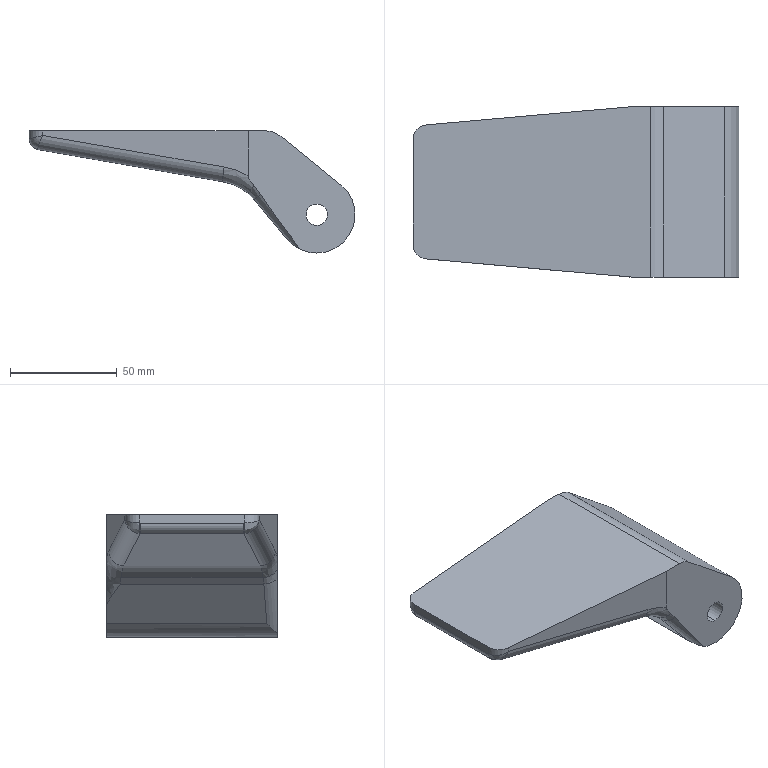Part | SolidWorks | features Extrusion 1, Fillet 1, ICE 1 | 1 solid | 29 faces | box 153 x 80 x 57.284 mm | volume 267395 mm3 | cylinder 11 | plane 9 | spline 9 | commonest cylinder face diameters 14 x5 10 x3 36 x2 50 x1